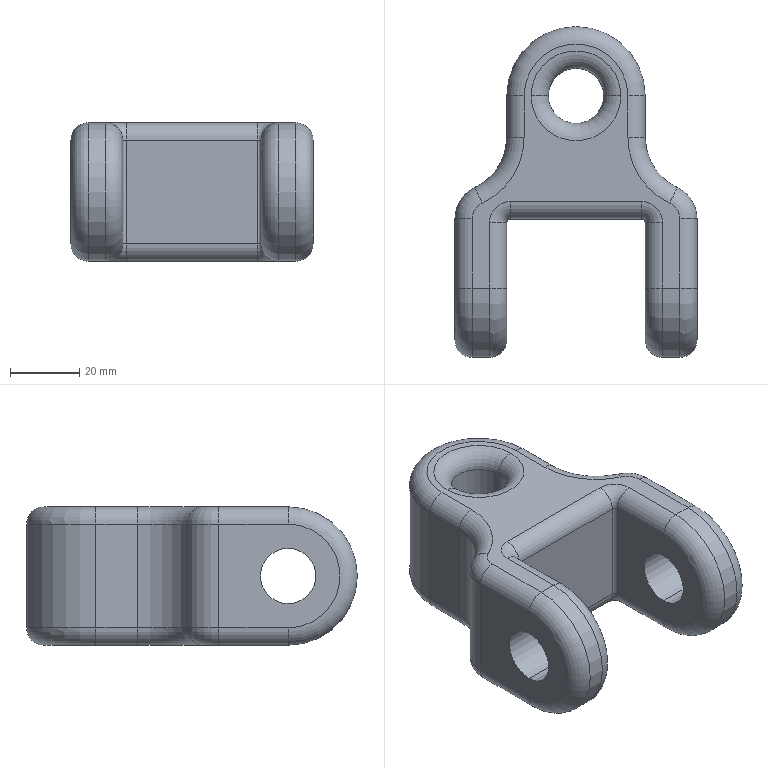Part | SolidWorks | 1 solid | 58 faces | box 70 x 95.558 x 40 mm | volume 119109 mm3 | cylinder 29 | torus 20 | plane 9 | commonest cylinder face diameters 10 x14 16 x6 40 x3 2 x2 20 x2 32 x2